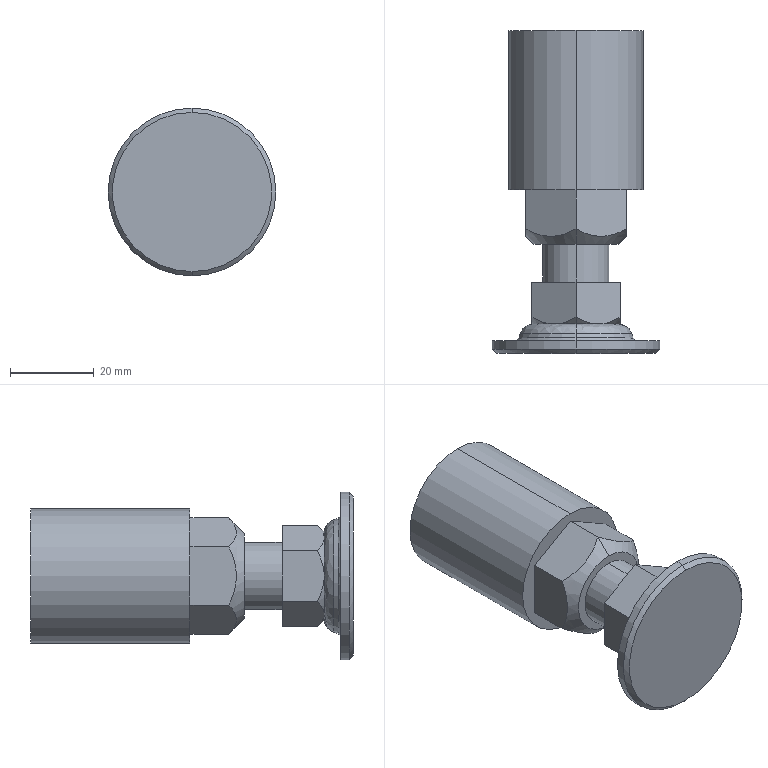Part | STEP file | CDAN75-Ma | 1 solid | 42 faces | box 40 x 77 x 40 mm | volume 48272 mm3 | plane 19 | cone 13 | cylinder 6 | spline 4 | commonest cylinder face diameters 16 x2 32 x2 40 x2